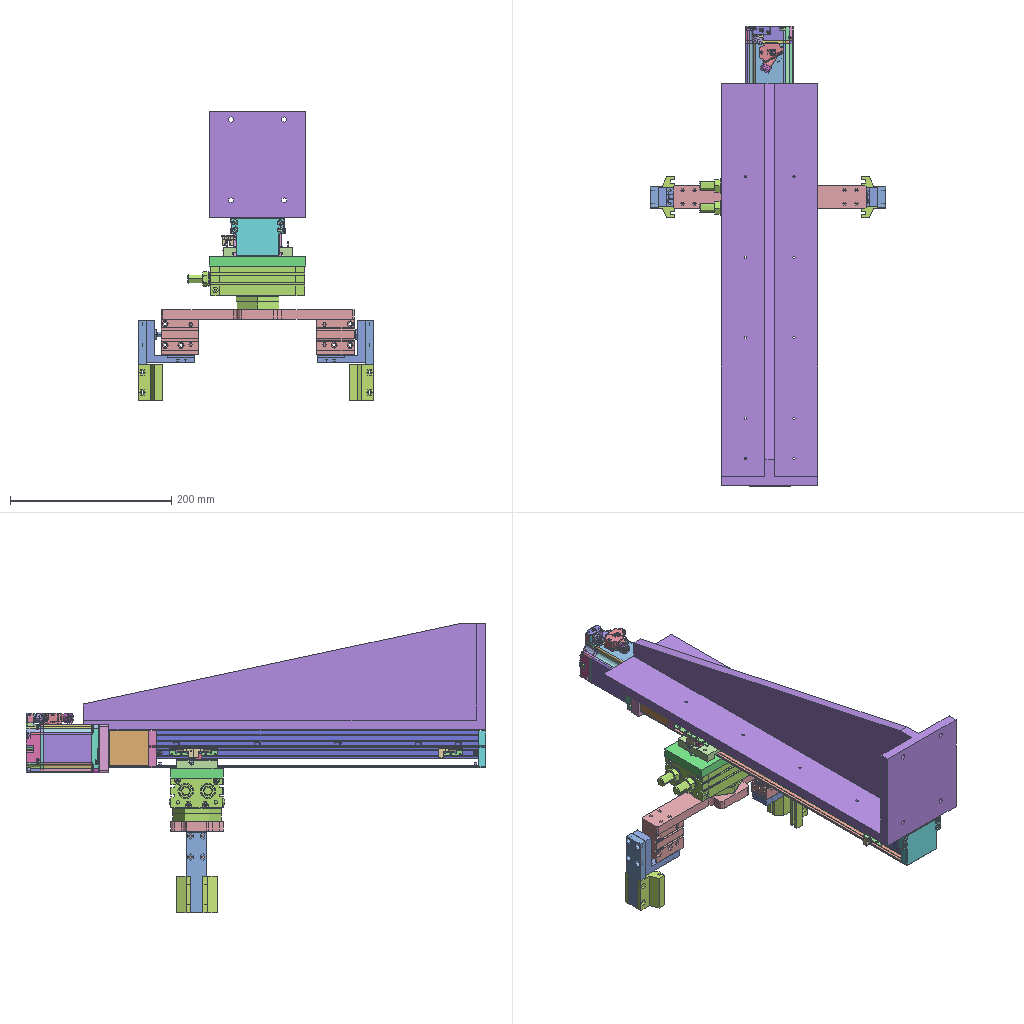Assembly | SolidWorks | 29 different items | 59 placed | box 292 x 571 x 359 mm
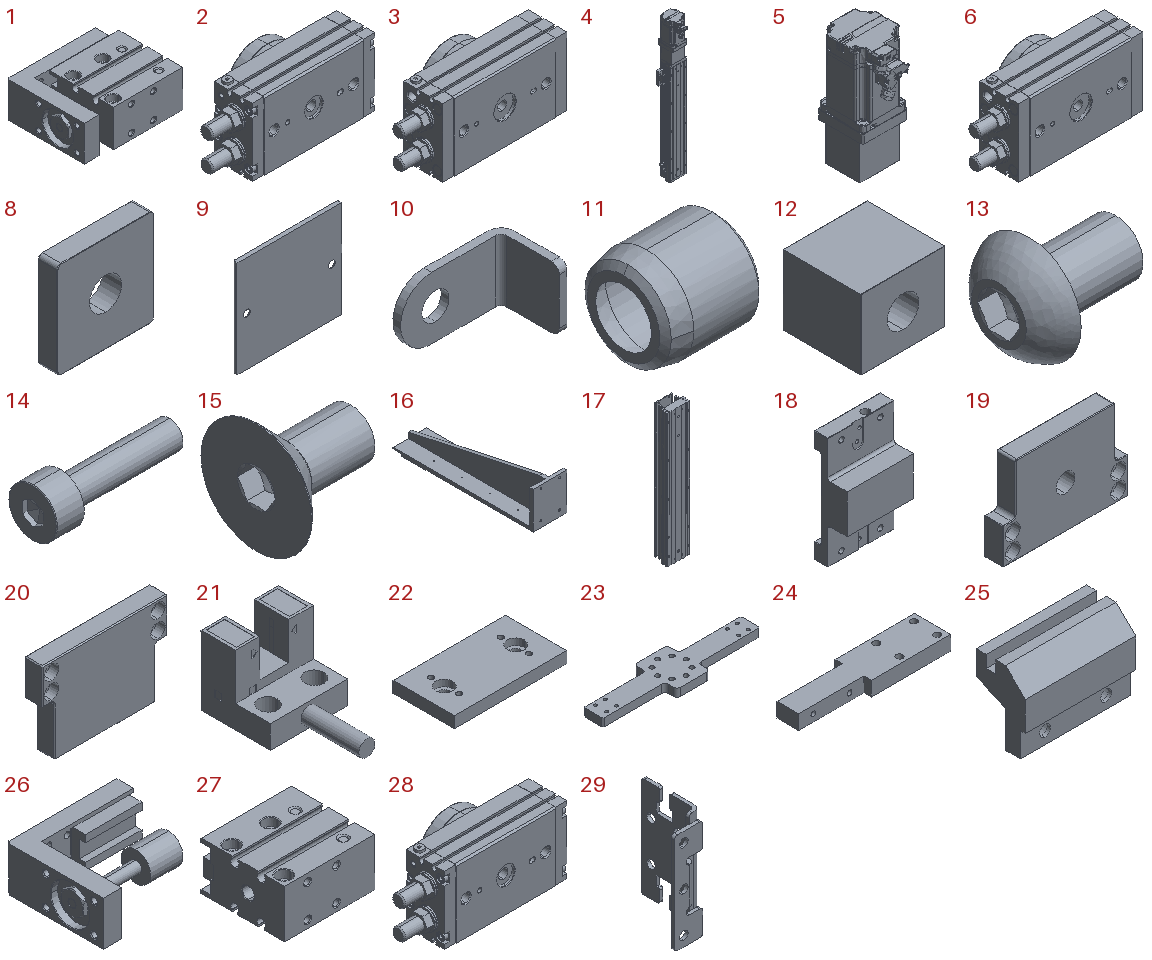Parts list (item | name | quantity | parent item | size | volume | features):
1 | (subassembly) | x2 | - | 66 x 53.5 x 25 mm | 64012 mm3 | -
2 | (subassembly) | x1 | - | 145.3 x 54 x 69 mm | 311465 mm3 | -
3 | (subassembly) | x1 | - | 154.5 x 57 x 74 mm | 391417 mm3 | -
4 | (subassembly) | x1 | - | - | - | -
5 | (subassembly) | x1 | in 4 | - | - | -
6 | - | x1 | - | 154.5 x 57 x 74 mm | 391417 mm3 | features BaseBody 1
7 | - | x1 | in 5 | - | - | features RefSurface 669
8 | - | x1 | in 5 | 60 x 12 x 60 mm | 39345 mm3 | features BaseBody 1
9 | - | x1 | in 5 | 53 x 2 x 49 mm | 5090 mm3 | features BaseBody 1
10 | - | x2 | in 4 | 14 x 8.5 x 8 mm | 150.836 mm3 | features BaseBody 1
11 | - | x2 | in 4 | 6.5 x 6.04 x 6.04 mm | 46.835 mm3 | features BaseBody 2
12 | - | x1 | in 5 | 53 x 49.2 x 44 mm | 99275 mm3 | features BaseBody 1
13 | - | x6 | in 4 | 6.65 x 5.7 x 5.7 mm | 59.694 mm3 | features BaseBody 1
14 | - | x8 | in 4 | 20 x 7 x 7 mm | 348.346 mm3 | features BaseBody 1
15 | - | x6 | in 4, 5 | 6 x 6.72 x 6.72 mm | 61.288 mm3 | features BaseBody 1
16 | - | x1 | - | 120 x 500 x 132 mm | 1285339 mm3 | features HoleWzd 3, ICE 2, Cut 1, Extrusion 1
17 | - | x1 | in 4 | 68 x 47 x 400 mm | 601851 mm3 | features BaseBody 2
18 | - | x1 | in 4 | 51 x 25.5 x 86 mm | 51756 mm3 | features BaseBody 1
19 | - | x1 | in 4 | 66 x 10 x 46 mm | 24787 mm3 | features BaseBody 1
20 | - | x1 | in 4 | 66 x 9 x 46 mm | 23009 mm3 | features BaseBody 1
21 | - | x3 | in 4 | 13.4 x 22 x 12 mm | 1082 mm3 | features BaseBody 1
22 | - | x1 | - | 120 x 65 x 12 mm | 86698 mm3 | features HoleWzd 2, Extrusion 1
23 | - | x1 | - | 240 x 65 x 12 mm | 96904 mm3 | features HoleWzd 2, Chamfer 1, Extrusion 1, Fillet 1, ICE 1, MirrorPattern 1
24 | - | x2 | - | 100 x 25 x 10 mm | 18975 mm3 | features HoleWzd 2, Cut 1, Extrusion 1
25 | - | x4 | - | 45 x 20 x 30 mm | 13803 mm3 | features ICE 2, Chamfer 1, Extrusion 1, HoleWzd 1
26 | - | x2 | in 1 | 60 x 52.5 x 24 mm | 27442 mm3 | features BaseBody 1
27 | - | x2 | in 1 | 47 x 43.5 x 25 mm | 36569 mm3 | features BaseBody 1
28 | - | x1 | in 2 | 145.3 x 54 x 69 mm | 311465 mm3 | features BaseBody 1
29 | - | x3 | in 4 | 11.322 x 20.322 x 30 mm | 726.14 mm3 | features BaseBody 1
Mates (type | each side: item.copy, entity, surface, feature):
In the top assembly
Coincident | 16.1 face plane Boss-Extrude1 | 17.1 face plane Input2
Width | 16.1 face plane Boss-Extrude1 | 16.1 face plane Boss-Extrude1 | 20.1 face plane Input1 | 20.1 face plane Input1
Coincident | 16.1 face plane Boss-Extrude1 | 20.1 face plane Input1
Coincident | 18.1 face plane Input1 | 22.1 face plane Boss-Extrude1
Width | 22.1 face plane Boss-Extrude1 | 22.1 face plane Boss-Extrude1 | 18.1 face plane Input1 | 18.1 face plane Input1 | 2 times
Coincident | 22.1 face plane Boss-Extrude1 | 28.1 face plane Input1
Width | 22.1 face plane Boss-Extrude1 | 22.1 face plane Boss-Extrude1 | 28.1 face plane Input1 | 28.1 face plane Input1 | 2 times
Coincident | 23.1 face plane Boss-Extrude1 | 28.1 face plane Input1
Coincident | 23.1 face plane Boss-Extrude1 | 27.1 face plane Input1 | 2 times
Width | 23.1 face plane Boss-Extrude1 | 23.1 face plane Boss-Extrude1 | 27.1 face plane Input1 | 27.1 face plane Input1
Width | 23.1 face plane Cut-Extrude1 | 23.1 face plane Cut-Extrude1 | 28.1 face cylinder Input1
Width | 23.1 face plane Boss-Extrude1 | 23.1 face plane Boss-Extrude1 | 28.1 face cylinder Input1
Coincident | 23.1 face plane Boss-Extrude1 | 27.2 face plane Input1 | 2 times
Coincident | 27.1 face plane Input1 | 27.2 face plane Input1
Coincident | 26.1 face plane Input1 | 24.1 face plane Boss-Extrude1 | 2 times
Width | 24.1 face plane Boss-Extrude1 | 24.1 face plane Boss-Extrude1 | 26.1 face plane Input1 | 26.1 face plane Input1
Coincident | 26.2 face plane Input1 | 24.2 face plane Boss-Extrude1
Width | 24.2 face plane Boss-Extrude1 | 24.2 face plane Boss-Extrude1 | 26.2 face plane Input1 | 26.2 face plane Input1
Coincident | 24.1 face plane Boss-Extrude1 | 24.2 face plane Boss-Extrude1
Coincident | 24.1 face plane Cut-Extrude1 | 25.1 face plane Boss-Extrude1
Coincident | 24.1 face plane Boss-Extrude1 | 25.1 face plane Boss-Extrude1
Coincident | 25.1 face plane Boss-Extrude1 | 25.2 face plane Boss-Extrude1 | 2 times
Coincident | 24.1 face plane Cut-Extrude1 | 25.1 face plane Cut-Extrude2
Coincident | 24.1 face plane Cut-Extrude1 | 25.2 face plane Cut-Extrude2
Coincident | 24.2 face plane Cut-Extrude1 | 25.3 face plane Cut-Extrude2
Coincident | 24.2 face plane Boss-Extrude1 | 25.3 face plane Boss-Extrude1 | 2 times
Coincident | 24.2 face plane Cut-Extrude1 | 25.4 face plane Cut-Extrude2
Coincident | 24.2 face plane Boss-Extrude1 | 25.4 face plane Boss-Extrude1 | 2 times
Parallel | 23.1 face plane Boss-Extrude1 | 28.1 face plane Input1
In subassembly 1
Concentric | 27.3 face cylinder Input1 | 26.3 face cylinder Input1
Parallel | 27.3 face plane Input1 | 26.3 face plane Input1
LimitDistanceDim | 26.3 face plane Input1 | 27.3 face plane Input1